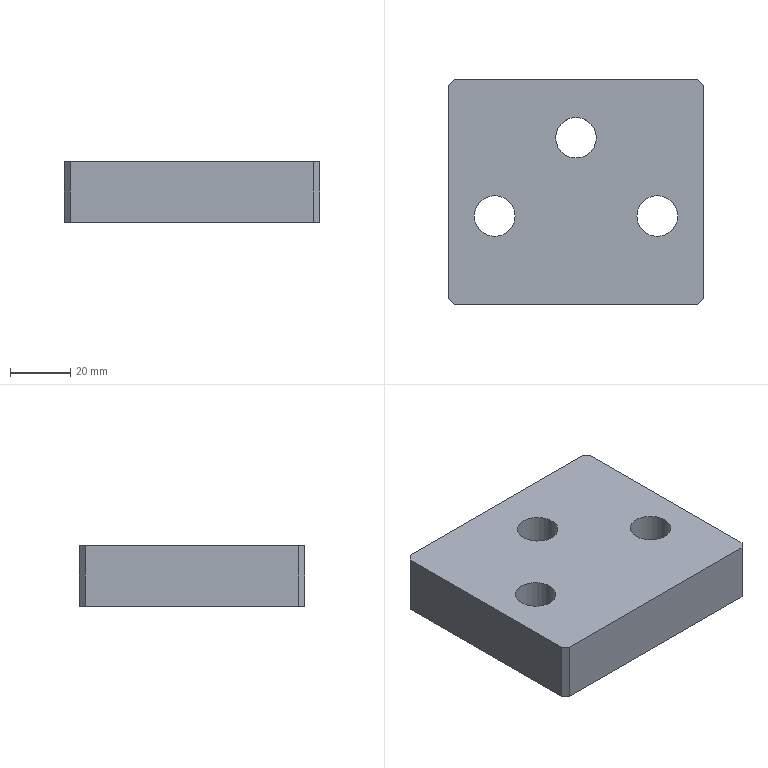Part | STEP file | lll_id1794_x_t | 1 solid | 13 faces | box 85 x 75 x 20 mm | volume 118740 mm3 | plane 10 | cylinder 3 | commonest cylinder face diameters 13.509 x3
STEP:
#1=CARTESIAN_POINT('',(2189.935,423.,-22.5));
#2=VERTEX_POINT('',#1);
#3=CARTESIAN_POINT('',(2189.935,352.,-22.5));
#4=VERTEX_POINT('',#3);
#5=CARTESIAN_POINT('',(2189.935,409.5,-22.5));
#6=DIRECTION('',(0.,-1.,0.));
#7=VECTOR('',#6,1.);
#8=LINE('',#5,#7);
#9=EDGE_CURVE('',#2,#4,#8,.T.);
#10=ORIENTED_EDGE('',*,*,#9,.T.);
#11=CARTESIAN_POINT('',(2187.935,350.,-22.5));
#12=VERTEX_POINT('',#11);
#13=CARTESIAN_POINT('',(2187.935,350.,-22.5));
#14=DIRECTION('',(0.7071,0.7071,0.));
#15=VECTOR('',#14,1.);
#16=LINE('',#13,#15);
#17=EDGE_CURVE('',#12,#4,#16,.T.);
#18=ORIENTED_EDGE('',*,*,#17,.F.);
#19=CARTESIAN_POINT('',(2106.935,350.,-22.5));
#20=VERTEX_POINT('',#19);
#21=CARTESIAN_POINT('',(2178.435,350.,-22.5));
#22=DIRECTION('',(-1.,0.,0.));
#23=VECTOR('',#22,1.);
#24=LINE('',#21,#23);
#25=EDGE_CURVE('',#12,#20,#24,.T.);
#26=ORIENTED_EDGE('',*,*,#25,.T.);
#27=CARTESIAN_POINT('',(2104.935,352.,-22.5));
#28=VERTEX_POINT('',#27);
#29=CARTESIAN_POINT('',(2104.935,352.,-22.5));
#30=DIRECTION('',(0.7071,-0.7071,0.));
#31=VECTOR('',#30,1.);
#32=LINE('',#29,#31);
#33=EDGE_CURVE('',#28,#20,#32,.T.);
#34=ORIENTED_EDGE('',*,*,#33,.F.);
#35=CARTESIAN_POINT('',(2104.935,423.,-22.5));
#36=VERTEX_POINT('',#35);
#37=CARTESIAN_POINT('',(2104.935,360.5,-22.5));
#38=DIRECTION('',(0.,1.,0.));
#39=VECTOR('',#38,1.);
#40=LINE('',#37,#39);
#41=EDGE_CURVE('',#28,#36,#40,.T.);
#42=ORIENTED_EDGE('',*,*,#41,.T.);
#43=CARTESIAN_POINT('',(2106.935,425.,-22.5));
#44=VERTEX_POINT('',#43);
#45=CARTESIAN_POINT('',(2106.935,425.,-22.5));
#46=DIRECTION('',(-0.7071,-0.7071,0.));
#47=VECTOR('',#46,1.);
#48=LINE('',#45,#47);
#49=EDGE_CURVE('',#44,#36,#48,.T.);
#50=ORIENTED_EDGE('',*,*,#49,.F.);
#51=CARTESIAN_POINT('',(2187.935,425.,-22.5));
#52=VERTEX_POINT('',#51);
#53=CARTESIAN_POINT('',(2126.435,425.,-22.5));
#54=DIRECTION('',(1.,0.,0.));
#55=VECTOR('',#54,1.);
#56=LINE('',#53,#55);
#57=EDGE_CURVE('',#44,#52,#56,.T.);
#58=ORIENTED_EDGE('',*,*,#57,.T.);
#59=CARTESIAN_POINT('',(2189.935,423.,-22.5));
#60=DIRECTION('',(-0.7071,0.7071,0.));
#61=VECTOR('',#60,1.);
#62=LINE('',#59,#61);
#63=EDGE_CURVE('',#2,#52,#62,.T.);
#64=ORIENTED_EDGE('',*,*,#63,.F.);
#65=EDGE_LOOP('',(#10,#18,#26,#34,#42,#50,#58,#64));
#66=FACE_BOUND('',#65,.T.);
#67=CARTESIAN_POINT('',(2140.681,405.5,-22.5));
#68=VERTEX_POINT('',#67);
#69=CARTESIAN_POINT('',(2147.435,405.5,-22.5));
#70=DIRECTION('',(0.,0.,-1.));
#71=DIRECTION('',(-1.,0.,0.));
#72=AXIS2_PLACEMENT_3D('',#69,#70,#71);
#73=CIRCLE('',#72,6.755);
#74=EDGE_CURVE('',#68,#68,#73,.T.);
#75=ORIENTED_EDGE('',*,*,#74,.F.);
#76=EDGE_LOOP('',(#75));
#77=FACE_BOUND('',#76,.T.);
#78=CARTESIAN_POINT('',(2113.681,379.5,-22.5));
#79=VERTEX_POINT('',#78);
#80=CARTESIAN_POINT('',(2120.435,379.5,-22.5));
#81=DIRECTION('',(0.,0.,1.));
#82=DIRECTION('',(-1.,0.,0.));
#83=AXIS2_PLACEMENT_3D('',#80,#81,#82);
#84=CIRCLE('',#83,6.755);
#85=EDGE_CURVE('',#79,#79,#84,.T.);
#86=ORIENTED_EDGE('',*,*,#85,.T.);
#87=EDGE_LOOP('',(#86));
#88=FACE_BOUND('',#87,.T.);
#89=CARTESIAN_POINT('',(2167.681,379.5,-22.5));
#90=VERTEX_POINT('',#89);
#91=CARTESIAN_POINT('',(2174.435,379.5,-22.5));
#92=DIRECTION('',(0.,0.,-1.));
#93=DIRECTION('',(-1.,0.,0.));
#94=AXIS2_PLACEMENT_3D('',#91,#92,#93);
#95=CIRCLE('',#94,6.755);
#96=EDGE_CURVE('',#90,#90,#95,.T.);
#97=ORIENTED_EDGE('',*,*,#96,.F.);
#98=EDGE_LOOP('',(#97));
#99=FACE_BOUND('',#98,.T.);
#100=CARTESIAN_POINT('',(2181.435,357.5,-22.5));
#101=DIRECTION('',(0.,0.,1.));
#102=DIRECTION('',(1.,0.,0.));
#103=AXIS2_PLACEMENT_3D('',#100,#101,#102);
#104=PLANE('',#103);
#105=ADVANCED_FACE('',(#66,#77,#88,#99),#104,.F.);
#106=CARTESIAN_POINT('',(2167.681,379.5,-2.5));
#107=VERTEX_POINT('',#106);
#108=CARTESIAN_POINT('',(2174.435,379.5,-2.5));
#109=DIRECTION('',(0.,0.,-1.));
#110=DIRECTION('',(-1.,0.,0.));
#111=AXIS2_PLACEMENT_3D('',#108,#109,#110);
#112=CIRCLE('',#111,6.755);
#113=EDGE_CURVE('',#107,#107,#112,.T.);
#114=ORIENTED_EDGE('',*,*,#113,.F.);
#115=EDGE_LOOP('',(#114));
#116=FACE_BOUND('',#115,.T.);
#117=ORIENTED_EDGE('',*,*,#96,.T.);
#118=EDGE_LOOP('',(#117));
#119=FACE_BOUND('',#118,.T.);
#120=CARTESIAN_POINT('',(2174.435,379.5,165.5));
#121=DIRECTION('',(0.,0.,-1.));
#122=DIRECTION('',(-1.,0.,0.));
#123=AXIS2_PLACEMENT_3D('',#120,#121,#122);
#124=CYLINDRICAL_SURFACE('',#123,6.755);
#125=ADVANCED_FACE('',(#116,#119),#124,.F.);
#126=CARTESIAN_POINT('',(2140.681,405.5,-2.5));
#127=VERTEX_POINT('',#126);
#128=CARTESIAN_POINT('',(2147.435,405.5,-2.5));
#129=DIRECTION('',(0.,0.,-1.));
#130=DIRECTION('',(-1.,0.,0.));
#131=AXIS2_PLACEMENT_3D('',#128,#129,#130);
#132=CIRCLE('',#131,6.755);
#133=EDGE_CURVE('',#127,#127,#132,.T.);
#134=ORIENTED_EDGE('',*,*,#133,.F.);
#135=EDGE_LOOP('',(#134));
#136=FACE_BOUND('',#135,.T.);
#137=ORIENTED_EDGE('',*,*,#74,.T.);
#138=EDGE_LOOP('',(#137));
#139=FACE_BOUND('',#138,.T.);
#140=CARTESIAN_POINT('',(2147.435,405.5,165.5));
#141=DIRECTION('',(0.,0.,-1.));
#142=DIRECTION('',(-1.,0.,0.));
#143=AXIS2_PLACEMENT_3D('',#140,#141,#142);
#144=CYLINDRICAL_SURFACE('',#143,6.755);
#145=ADVANCED_FACE('',(#136,#139),#144,.F.);
#146=ORIENTED_EDGE('',*,*,#57,.F.);
#147=CARTESIAN_POINT('',(2106.935,425.,-2.5));
#148=VERTEX_POINT('',#147);
#149=CARTESIAN_POINT('',(2106.935,425.,-2.5));
#150=DIRECTION('',(0.,0.,-1.));
#151=VECTOR('',#150,1.);
#152=LINE('',#149,#151);
#153=EDGE_CURVE('',#148,#44,#152,.T.);
#154=ORIENTED_EDGE('',*,*,#153,.F.);
#155=CARTESIAN_POINT('',(2187.935,425.,-2.5));
#156=VERTEX_POINT('',#155);
#157=CARTESIAN_POINT('',(2126.435,425.,-2.5));
#158=DIRECTION('',(1.,0.,0.));
#159=VECTOR('',#158,1.);
#160=LINE('',#157,#159);
#161=EDGE_CURVE('',#148,#156,#160,.T.);
#162=ORIENTED_EDGE('',*,*,#161,.T.);
#163=CARTESIAN_POINT('',(2187.935,425.,-2.5));
#164=DIRECTION('',(0.,0.,1.));
#165=VECTOR('',#164,1.);
#166=LINE('',#163,#165);
#167=EDGE_CURVE('',#52,#156,#166,.T.);
#168=ORIENTED_EDGE('',*,*,#167,.F.);
#169=EDGE_LOOP('',(#146,#154,#162,#168));
#170=FACE_OUTER_BOUND('',#169,.T.);
#171=CARTESIAN_POINT('',(2126.435,425.,-2.5));
#172=DIRECTION('',(0.,-1.,0.));
#173=DIRECTION('',(0.,0.,1.));
#174=AXIS2_PLACEMENT_3D('',#171,#172,#173);
#175=PLANE('',#174);
#176=ADVANCED_FACE('',(#170),#175,.F.);
#177=CARTESIAN_POINT('',(2104.935,352.,-2.5));
#178=VERTEX_POINT('',#177);
#179=CARTESIAN_POINT('',(2104.935,423.,-2.5));
#180=VERTEX_POINT('',#179);
#181=CARTESIAN_POINT('',(2104.935,360.5,-2.5));
#182=DIRECTION('',(0.,1.,0.));
#183=VECTOR('',#182,1.);
#184=LINE('',#181,#183);
#185=EDGE_CURVE('',#178,#180,#184,.T.);
#186=ORIENTED_EDGE('',*,*,#185,.T.);
#187=CARTESIAN_POINT('',(2104.935,423.,-2.5));
#188=DIRECTION('',(0.,0.,1.));
#189=VECTOR('',#188,1.);
#190=LINE('',#187,#189);
#191=EDGE_CURVE('',#36,#180,#190,.T.);
#192=ORIENTED_EDGE('',*,*,#191,.F.);
#193=ORIENTED_EDGE('',*,*,#41,.F.);
#194=CARTESIAN_POINT('',(2104.935,352.,-2.5));
#195=DIRECTION('',(0.,0.,-1.));
#196=VECTOR('',#195,1.);
#197=LINE('',#194,#196);
#198=EDGE_CURVE('',#178,#28,#197,.T.);
#199=ORIENTED_EDGE('',*,*,#198,.F.);
#200=EDGE_LOOP('',(#186,#192,#193,#199));
#201=FACE_OUTER_BOUND('',#200,.T.);
#202=CARTESIAN_POINT('',(2104.935,360.5,-2.5));
#203=DIRECTION('',(1.,0.,0.));
#204=DIRECTION('',(0.,0.,-1.));
#205=AXIS2_PLACEMENT_3D('',#202,#203,#204);
#206=PLANE('',#205);
#207=ADVANCED_FACE('',(#201),#206,.F.);
#208=CARTESIAN_POINT('',(2187.935,350.,-2.5));
#209=VERTEX_POINT('',#208);
#210=CARTESIAN_POINT('',(2106.935,350.,-2.5));
#211=VERTEX_POINT('',#210);
#212=CARTESIAN_POINT('',(2178.435,350.,-2.5));
#213=DIRECTION('',(-1.,0.,0.));
#214=VECTOR('',#213,1.);
#215=LINE('',#212,#214);
#216=EDGE_CURVE('',#209,#211,#215,.T.);
#217=ORIENTED_EDGE('',*,*,#216,.T.);
#218=CARTESIAN_POINT('',(2106.935,350.,-2.5));
#219=DIRECTION('',(0.,0.,1.));
#220=VECTOR('',#219,1.);
#221=LINE('',#218,#220);
#222=EDGE_CURVE('',#20,#211,#221,.T.);
#223=ORIENTED_EDGE('',*,*,#222,.F.);
#224=ORIENTED_EDGE('',*,*,#25,.F.);
#225=CARTESIAN_POINT('',(2187.935,350.,-2.5));
#226=DIRECTION('',(0.,0.,-1.));
#227=VECTOR('',#226,1.);
#228=LINE('',#225,#227);
#229=EDGE_CURVE('',#209,#12,#228,.T.);
#230=ORIENTED_EDGE('',*,*,#229,.F.);
#231=EDGE_LOOP('',(#217,#223,#224,#230));
#232=FACE_OUTER_BOUND('',#231,.T.);
#233=CARTESIAN_POINT('',(2178.435,350.,-2.5));
#234=DIRECTION('',(0.,1.,0.));
#235=DIRECTION('',(0.,0.,-1.));
#236=AXIS2_PLACEMENT_3D('',#233,#234,#235);
#237=PLANE('',#236);
#238=ADVANCED_FACE('',(#232),#237,.F.);
#239=CARTESIAN_POINT('',(2189.935,423.,-2.5));
#240=VERTEX_POINT('',#239);
#241=CARTESIAN_POINT('',(2189.935,352.,-2.5));
#242=VERTEX_POINT('',#241);
#243=CARTESIAN_POINT('',(2189.935,409.5,-2.5));
#244=DIRECTION('',(0.,-1.,0.));
#245=VECTOR('',#244,1.);
#246=LINE('',#243,#245);
#247=EDGE_CURVE('',#240,#242,#246,.T.);
#248=ORIENTED_EDGE('',*,*,#247,.T.);
#249=CARTESIAN_POINT('',(2189.935,352.,-2.5));
#250=DIRECTION('',(0.,0.,1.));
#251=VECTOR('',#250,1.);
#252=LINE('',#249,#251);
#253=EDGE_CURVE('',#4,#242,#252,.T.);
#254=ORIENTED_EDGE('',*,*,#253,.F.);
#255=ORIENTED_EDGE('',*,*,#9,.F.);
#256=CARTESIAN_POINT('',(2189.935,423.,-2.5));
#257=DIRECTION('',(0.,0.,-1.));
#258=VECTOR('',#257,1.);
#259=LINE('',#256,#258);
#260=EDGE_CURVE('',#240,#2,#259,.T.);
#261=ORIENTED_EDGE('',*,*,#260,.F.);
#262=EDGE_LOOP('',(#248,#254,#255,#261));
#263=FACE_OUTER_BOUND('',#262,.T.);
#264=CARTESIAN_POINT('',(2189.935,409.5,-2.5));
#265=DIRECTION('',(-1.,0.,0.));
#266=DIRECTION('',(0.,0.,1.));
#267=AXIS2_PLACEMENT_3D('',#264,#265,#266);
#268=PLANE('',#267);
#269=ADVANCED_FACE('',(#263),#268,.F.);
#270=ORIENTED_EDGE('',*,*,#113,.T.);
#271=EDGE_LOOP('',(#270));
#272=FACE_BOUND('',#271,.T.);
#273=ORIENTED_EDGE('',*,*,#161,.F.);
#274=CARTESIAN_POINT('',(2105.435,423.5,-2.5));
#275=DIRECTION('',(0.7071,0.7071,0.));
#276=VECTOR('',#275,1.);
#277=LINE('',#274,#276);
#278=EDGE_CURVE('',#180,#148,#277,.T.);
#279=ORIENTED_EDGE('',*,*,#278,.F.);
#280=ORIENTED_EDGE('',*,*,#185,.F.);
#281=CARTESIAN_POINT('',(2132.935,324.,-2.5));
#282=DIRECTION('',(-0.7071,0.7071,0.));
#283=VECTOR('',#282,1.);
#284=LINE('',#281,#283);
#285=EDGE_CURVE('',#211,#178,#284,.T.);
#286=ORIENTED_EDGE('',*,*,#285,.F.);
#287=ORIENTED_EDGE('',*,*,#216,.F.);
#288=CARTESIAN_POINT('',(2190.935,353.,-2.5));
#289=DIRECTION('',(-0.7071,-0.7071,0.));
#290=VECTOR('',#289,1.);
#291=LINE('',#288,#290);
#292=EDGE_CURVE('',#242,#209,#291,.T.);
#293=ORIENTED_EDGE('',*,*,#292,.F.);
#294=ORIENTED_EDGE('',*,*,#247,.F.);
#295=CARTESIAN_POINT('',(2218.435,394.5,-2.5));
#296=DIRECTION('',(0.7071,-0.7071,0.));
#297=VECTOR('',#296,1.);
#298=LINE('',#295,#297);
#299=EDGE_CURVE('',#156,#240,#298,.T.);
#300=ORIENTED_EDGE('',*,*,#299,.F.);
#301=EDGE_LOOP('',(#273,#279,#280,#286,#287,#293,#294,#300));
#302=FACE_BOUND('',#301,.T.);
#303=ORIENTED_EDGE('',*,*,#133,.T.);
#304=EDGE_LOOP('',(#303));
#305=FACE_BOUND('',#304,.T.);
#306=CARTESIAN_POINT('',(2113.681,379.5,-2.5));
#307=VERTEX_POINT('',#306);
#308=CARTESIAN_POINT('',(2120.435,379.5,-2.5));
#309=DIRECTION('',(0.,0.,-1.));
#310=DIRECTION('',(-1.,0.,0.));
#311=AXIS2_PLACEMENT_3D('',#308,#309,#310);
#312=CIRCLE('',#311,6.755);
#313=EDGE_CURVE('',#307,#307,#312,.T.);
#314=ORIENTED_EDGE('',*,*,#313,.T.);
#315=EDGE_LOOP('',(#314));
#316=FACE_BOUND('',#315,.T.);
#317=CARTESIAN_POINT('',(2181.435,357.5,-2.5));
#318=DIRECTION('',(0.,0.,1.));
#319=DIRECTION('',(1.,0.,0.));
#320=AXIS2_PLACEMENT_3D('',#317,#318,#319);
#321=PLANE('',#320);
#322=ADVANCED_FACE('',(#272,#302,#305,#316),#321,.T.);
#323=ORIENTED_EDGE('',*,*,#85,.F.);
#324=EDGE_LOOP('',(#323));
#325=FACE_BOUND('',#324,.T.);
#326=ORIENTED_EDGE('',*,*,#313,.F.);
#327=EDGE_LOOP('',(#326));
#328=FACE_BOUND('',#327,.T.);
#329=CARTESIAN_POINT('',(2120.435,379.5,165.5));
#330=DIRECTION('',(0.,0.,-1.));
#331=DIRECTION('',(-1.,0.,0.));
#332=AXIS2_PLACEMENT_3D('',#329,#330,#331);
#333=CYLINDRICAL_SURFACE('',#332,6.755);
#334=ADVANCED_FACE('',(#325,#328),#333,.F.);
#335=ORIENTED_EDGE('',*,*,#299,.T.);
#336=ORIENTED_EDGE('',*,*,#260,.T.);
#337=ORIENTED_EDGE('',*,*,#63,.T.);
#338=ORIENTED_EDGE('',*,*,#167,.T.);
#339=EDGE_LOOP('',(#335,#336,#337,#338));
#340=FACE_OUTER_BOUND('',#339,.T.);
#341=CARTESIAN_POINT('',(2189.935,423.,-2.5));
#342=DIRECTION('',(-0.7071,-0.7071,0.));
#343=DIRECTION('',(0.,0.,-1.));
#344=AXIS2_PLACEMENT_3D('',#341,#342,#343);
#345=PLANE('',#344);
#346=ADVANCED_FACE('',(#340),#345,.F.);
#347=ORIENTED_EDGE('',*,*,#292,.T.);
#348=ORIENTED_EDGE('',*,*,#229,.T.);
#349=ORIENTED_EDGE('',*,*,#17,.T.);
#350=ORIENTED_EDGE('',*,*,#253,.T.);
#351=EDGE_LOOP('',(#347,#348,#349,#350));
#352=FACE_OUTER_BOUND('',#351,.T.);
#353=CARTESIAN_POINT('',(2187.935,350.,-2.5));
#354=DIRECTION('',(-0.7071,0.7071,0.));
#355=DIRECTION('',(0.,0.,-1.));
#356=AXIS2_PLACEMENT_3D('',#353,#354,#355);
#357=PLANE('',#356);
#358=ADVANCED_FACE('',(#352),#357,.F.);
#359=ORIENTED_EDGE('',*,*,#285,.T.);
#360=ORIENTED_EDGE('',*,*,#198,.T.);
#361=ORIENTED_EDGE('',*,*,#33,.T.);
#362=ORIENTED_EDGE('',*,*,#222,.T.);
#363=EDGE_LOOP('',(#359,#360,#361,#362));
#364=FACE_OUTER_BOUND('',#363,.T.);
#365=CARTESIAN_POINT('',(2104.935,352.,-2.5));
#366=DIRECTION('',(0.7071,0.7071,0.));
#367=DIRECTION('',(0.,0.,-1.));
#368=AXIS2_PLACEMENT_3D('',#365,#366,#367);
#369=PLANE('',#368);
#370=ADVANCED_FACE('',(#364),#369,.F.);
#371=ORIENTED_EDGE('',*,*,#278,.T.);
#372=ORIENTED_EDGE('',*,*,#153,.T.);
#373=ORIENTED_EDGE('',*,*,#49,.T.);
#374=ORIENTED_EDGE('',*,*,#191,.T.);
#375=EDGE_LOOP('',(#371,#372,#373,#374));
#376=FACE_OUTER_BOUND('',#375,.T.);
#377=CARTESIAN_POINT('',(2106.935,425.,-2.5));
#378=DIRECTION('',(0.7071,-0.7071,0.));
#379=DIRECTION('',(0.,0.,-1.));
#380=AXIS2_PLACEMENT_3D('',#377,#378,#379);
#381=PLANE('',#380);
#382=ADVANCED_FACE('',(#376),#381,.F.);
#383=CLOSED_SHELL('',(#105,#125,#145,#176,#207,#238,#269,#322,#334,#346,#358,#370,#382));
#384=MANIFOLD_SOLID_BREP('',#383);
#385=(LENGTH_UNIT()NAMED_UNIT(*)SI_UNIT(.MILLI.,.METRE.));
#386=UNCERTAINTY_MEASURE_WITH_UNIT(LENGTH_MEASURE(0.00002),#385,'','');
#387=(NAMED_UNIT(*)PLANE_ANGLE_UNIT()SI_UNIT($,.RADIAN.));
#388=PLANE_ANGLE_MEASURE_WITH_UNIT(PLANE_ANGLE_MEASURE(0.01745),#387);
#389=DIMENSIONAL_EXPONENTS(0.,0.,0.,0.,0.,0.,0.);
#390=(CONVERSION_BASED_UNIT('DEGREE',#388)NAMED_UNIT(#389)PLANE_ANGLE_UNIT());
#391=(NAMED_UNIT(*)SI_UNIT($,.STERADIAN.)SOLID_ANGLE_UNIT());
#392=(GEOMETRIC_REPRESENTATION_CONTEXT(3)GLOBAL_UNCERTAINTY_ASSIGNED_CONTEXT((#386))GLOBAL_UNIT_ASSIGNED_CONTEXT((#385,#390,#391))REPRESENTATION_CONTEXT('',''));
#393=ADVANCED_BREP_SHAPE_REPRESENTATION('',(#384),#392);